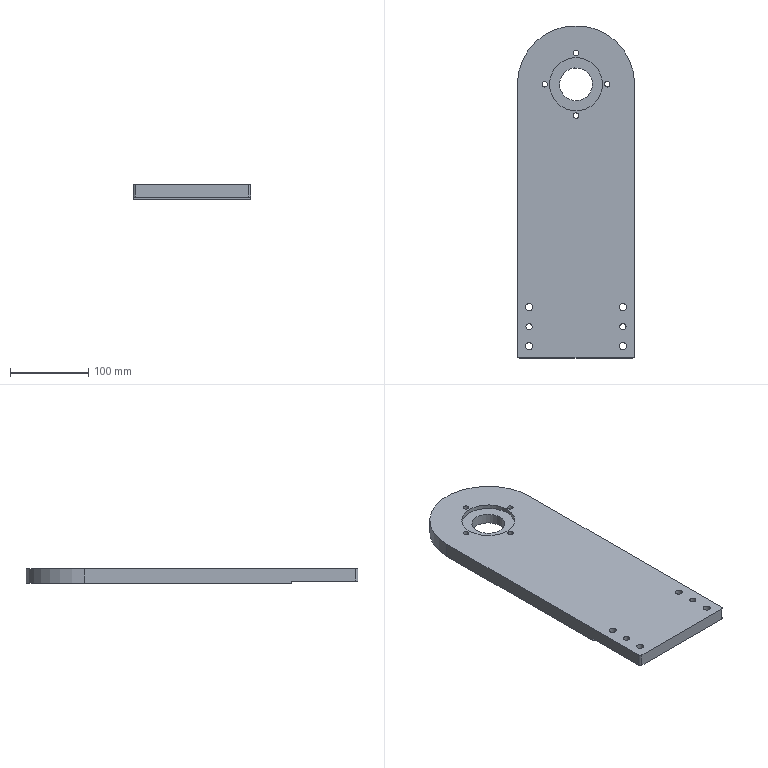Part | STEP file | SN10_010_006_PLACA | 1 solid | 23 faces | box 150 x 425 x 19 mm | volume 1079785 mm3 | cylinder 15 | plane 8 | commonest cylinder face diameters 7 x4 9 x4 6 x2 8 x2 42 x1 68 x1